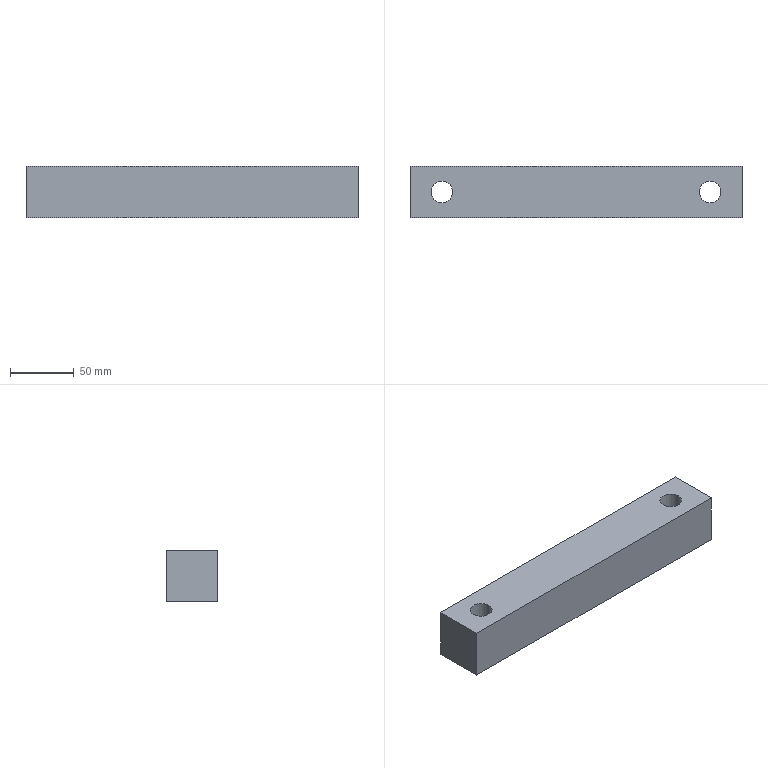Part | STEP file | 1 solid | 12 faces | box 260 x 40 x 40 mm | volume 385684 mm3 | plane 8 | cylinder 4 | commonest cylinder face diameters 17 x2 26 x2
STEP:
#1=CARTESIAN_POINT('',(3.,-262.5,-147.));
#2=VERTEX_POINT('',#1);
#3=CARTESIAN_POINT('',(-10.,-262.5,-147.));
#4=DIRECTION('',(0.,0.,-1.));
#5=DIRECTION('',(1.,0.,0.));
#6=AXIS2_PLACEMENT_3D('',#3,#4,#5);
#7=CIRCLE('',#6,13.);
#8=EDGE_CURVE('',#2,#2,#7,.T.);
#9=ORIENTED_EDGE('',*,*,#8,.F.);
#10=EDGE_LOOP('',(#9));
#11=FACE_BOUND('',#10,.T.);
#12=CARTESIAN_POINT('',(-233.,-262.5,-147.));
#13=VERTEX_POINT('',#12);
#14=CARTESIAN_POINT('',(-220.,-262.5,-147.));
#15=DIRECTION('',(0.,0.,1.));
#16=DIRECTION('',(-1.,0.,0.));
#17=AXIS2_PLACEMENT_3D('',#14,#15,#16);
#18=CIRCLE('',#17,13.);
#19=EDGE_CURVE('',#13,#13,#18,.T.);
#20=ORIENTED_EDGE('',*,*,#19,.T.);
#21=EDGE_LOOP('',(#20));
#22=FACE_BOUND('',#21,.T.);
#23=CARTESIAN_POINT('',(-245.,-282.5,-147.));
#24=VERTEX_POINT('',#23);
#25=CARTESIAN_POINT('',(15.,-282.5,-147.));
#26=VERTEX_POINT('',#25);
#27=CARTESIAN_POINT('',(25.,-282.5,-147.));
#28=DIRECTION('',(1.,0.,0.));
#29=VECTOR('',#28,1.);
#30=LINE('',#27,#29);
#31=EDGE_CURVE('',#24,#26,#30,.T.);
#32=ORIENTED_EDGE('',*,*,#31,.F.);
#33=CARTESIAN_POINT('',(-245.,-242.5,-147.));
#34=VERTEX_POINT('',#33);
#35=CARTESIAN_POINT('',(-245.,-262.5,-147.));
#36=DIRECTION('',(0.,-1.,0.));
#37=VECTOR('',#36,1.);
#38=LINE('',#35,#37);
#39=EDGE_CURVE('',#34,#24,#38,.T.);
#40=ORIENTED_EDGE('',*,*,#39,.F.);
#41=CARTESIAN_POINT('',(15.,-242.5,-147.));
#42=VERTEX_POINT('',#41);
#43=CARTESIAN_POINT('',(-22.5,-242.5,-147.));
#44=DIRECTION('',(1.,0.,0.));
#45=VECTOR('',#44,1.);
#46=LINE('',#43,#45);
#47=EDGE_CURVE('',#34,#42,#46,.T.);
#48=ORIENTED_EDGE('',*,*,#47,.T.);
#49=CARTESIAN_POINT('',(15.,-262.5,-147.));
#50=DIRECTION('',(0.,-1.,0.));
#51=VECTOR('',#50,1.);
#52=LINE('',#49,#51);
#53=EDGE_CURVE('',#42,#26,#52,.T.);
#54=ORIENTED_EDGE('',*,*,#53,.T.);
#55=EDGE_LOOP('',(#32,#40,#48,#54));
#56=FACE_BOUND('',#55,.T.);
#57=CARTESIAN_POINT('',(-115.,-262.5,-147.));
#58=DIRECTION('',(0.,0.,-1.));
#59=DIRECTION('',(-1.,0.,0.));
#60=AXIS2_PLACEMENT_3D('',#57,#58,#59);
#61=PLANE('',#60);
#62=ADVANCED_FACE('',(#11,#22,#56),#61,.T.);
#63=CARTESIAN_POINT('',(-1.5,-262.5,-107.));
#64=VERTEX_POINT('',#63);
#65=CARTESIAN_POINT('',(-10.,-262.5,-107.));
#66=DIRECTION('',(0.,0.,1.));
#67=DIRECTION('',(1.,0.,0.));
#68=AXIS2_PLACEMENT_3D('',#65,#66,#67);
#69=CIRCLE('',#68,8.5);
#70=EDGE_CURVE('',#64,#64,#69,.T.);
#71=ORIENTED_EDGE('',*,*,#70,.F.);
#72=EDGE_LOOP('',(#71));
#73=FACE_BOUND('',#72,.T.);
#74=CARTESIAN_POINT('',(-228.5,-262.5,-107.));
#75=VERTEX_POINT('',#74);
#76=CARTESIAN_POINT('',(-220.,-262.5,-107.));
#77=DIRECTION('',(0.,0.,-1.));
#78=DIRECTION('',(-1.,0.,0.));
#79=AXIS2_PLACEMENT_3D('',#76,#77,#78);
#80=CIRCLE('',#79,8.5);
#81=EDGE_CURVE('',#75,#75,#80,.T.);
#82=ORIENTED_EDGE('',*,*,#81,.T.);
#83=EDGE_LOOP('',(#82));
#84=FACE_BOUND('',#83,.T.);
#85=CARTESIAN_POINT('',(15.,-242.5,-107.));
#86=VERTEX_POINT('',#85);
#87=CARTESIAN_POINT('',(15.,-282.5,-107.));
#88=VERTEX_POINT('',#87);
#89=CARTESIAN_POINT('',(15.,9.,-107.));
#90=DIRECTION('',(0.,-1.,0.));
#91=VECTOR('',#90,1.);
#92=LINE('',#89,#91);
#93=EDGE_CURVE('',#86,#88,#92,.T.);
#94=ORIENTED_EDGE('',*,*,#93,.F.);
#95=CARTESIAN_POINT('',(-245.,-242.5,-107.));
#96=VERTEX_POINT('',#95);
#97=CARTESIAN_POINT('',(25.,-242.5,-107.));
#98=DIRECTION('',(1.,0.,0.));
#99=VECTOR('',#98,1.);
#100=LINE('',#97,#99);
#101=EDGE_CURVE('',#96,#86,#100,.T.);
#102=ORIENTED_EDGE('',*,*,#101,.F.);
#103=CARTESIAN_POINT('',(-245.,-282.5,-107.));
#104=VERTEX_POINT('',#103);
#105=CARTESIAN_POINT('',(-245.,-243.548,-107.));
#106=DIRECTION('',(0.,-1.,0.));
#107=VECTOR('',#106,1.);
#108=LINE('',#105,#107);
#109=EDGE_CURVE('',#96,#104,#108,.T.);
#110=ORIENTED_EDGE('',*,*,#109,.T.);
#111=CARTESIAN_POINT('',(25.,-282.5,-107.));
#112=DIRECTION('',(-1.,0.,0.));
#113=VECTOR('',#112,1.);
#114=LINE('',#111,#113);
#115=EDGE_CURVE('',#88,#104,#114,.T.);
#116=ORIENTED_EDGE('',*,*,#115,.F.);
#117=EDGE_LOOP('',(#94,#102,#110,#116));
#118=FACE_BOUND('',#117,.T.);
#119=CARTESIAN_POINT('',(25.,9.,-107.));
#120=DIRECTION('',(0.,0.,-1.));
#121=DIRECTION('',(0.,-1.,0.));
#122=AXIS2_PLACEMENT_3D('',#119,#120,#121);
#123=PLANE('',#122);
#124=ADVANCED_FACE('',(#73,#84,#118),#123,.F.);
#125=CARTESIAN_POINT('',(15.,-282.5,-107.));
#126=DIRECTION('',(0.,0.,1.));
#127=VECTOR('',#126,1.);
#128=LINE('',#125,#127);
#129=EDGE_CURVE('',#26,#88,#128,.T.);
#130=ORIENTED_EDGE('',*,*,#129,.F.);
#131=ORIENTED_EDGE('',*,*,#53,.F.);
#132=CARTESIAN_POINT('',(15.,-242.5,-199.5));
#133=DIRECTION('',(0.,0.,-1.));
#134=VECTOR('',#133,1.);
#135=LINE('',#132,#134);
#136=EDGE_CURVE('',#86,#42,#135,.T.);
#137=ORIENTED_EDGE('',*,*,#136,.F.);
#138=ORIENTED_EDGE('',*,*,#93,.T.);
#139=EDGE_LOOP('',(#130,#131,#137,#138));
#140=FACE_OUTER_BOUND('',#139,.T.);
#141=CARTESIAN_POINT('',(15.,9.,-107.));
#142=DIRECTION('',(-1.,0.,0.));
#143=DIRECTION('',(0.,-1.,0.));
#144=AXIS2_PLACEMENT_3D('',#141,#142,#143);
#145=PLANE('',#144);
#146=ADVANCED_FACE('',(#140),#145,.F.);
#147=ORIENTED_EDGE('',*,*,#39,.T.);
#148=CARTESIAN_POINT('',(-245.,-282.5,-107.));
#149=DIRECTION('',(0.,0.,1.));
#150=VECTOR('',#149,1.);
#151=LINE('',#148,#150);
#152=EDGE_CURVE('',#24,#104,#151,.T.);
#153=ORIENTED_EDGE('',*,*,#152,.T.);
#154=ORIENTED_EDGE('',*,*,#109,.F.);
#155=CARTESIAN_POINT('',(-245.,-242.5,-107.));
#156=DIRECTION('',(0.,0.,1.));
#157=VECTOR('',#156,1.);
#158=LINE('',#155,#157);
#159=EDGE_CURVE('',#34,#96,#158,.T.);
#160=ORIENTED_EDGE('',*,*,#159,.F.);
#161=EDGE_LOOP('',(#147,#153,#154,#160));
#162=FACE_OUTER_BOUND('',#161,.T.);
#163=CARTESIAN_POINT('',(-245.,-243.548,-107.));
#164=DIRECTION('',(1.,0.,0.));
#165=DIRECTION('',(0.,0.,1.));
#166=AXIS2_PLACEMENT_3D('',#163,#164,#165);
#167=PLANE('',#166);
#168=ADVANCED_FACE('',(#162),#167,.F.);
#169=ORIENTED_EDGE('',*,*,#152,.F.);
#170=ORIENTED_EDGE('',*,*,#31,.T.);
#171=ORIENTED_EDGE('',*,*,#129,.T.);
#172=ORIENTED_EDGE('',*,*,#115,.T.);
#173=EDGE_LOOP('',(#169,#170,#171,#172));
#174=FACE_OUTER_BOUND('',#173,.T.);
#175=CARTESIAN_POINT('',(25.,-282.5,-107.));
#176=DIRECTION('',(0.,1.,0.));
#177=DIRECTION('',(0.,0.,-1.));
#178=AXIS2_PLACEMENT_3D('',#175,#176,#177);
#179=PLANE('',#178);
#180=ADVANCED_FACE('',(#174),#179,.F.);
#181=ORIENTED_EDGE('',*,*,#136,.T.);
#182=ORIENTED_EDGE('',*,*,#47,.F.);
#183=ORIENTED_EDGE('',*,*,#159,.T.);
#184=ORIENTED_EDGE('',*,*,#101,.T.);
#185=EDGE_LOOP('',(#181,#182,#183,#184));
#186=FACE_OUTER_BOUND('',#185,.T.);
#187=CARTESIAN_POINT('',(-22.5,-242.5,-199.5));
#188=DIRECTION('',(0.,1.,0.));
#189=DIRECTION('',(0.,0.,1.));
#190=AXIS2_PLACEMENT_3D('',#187,#188,#189);
#191=PLANE('',#190);
#192=ADVANCED_FACE('',(#186),#191,.T.);
#193=CARTESIAN_POINT('',(-211.5,-262.5,-127.));
#194=VERTEX_POINT('',#193);
#195=CARTESIAN_POINT('',(-220.,-262.5,-127.));
#196=DIRECTION('',(0.,0.,1.));
#197=DIRECTION('',(1.,0.,0.));
#198=AXIS2_PLACEMENT_3D('',#195,#196,#197);
#199=CIRCLE('',#198,8.5);
#200=EDGE_CURVE('',#194,#194,#199,.T.);
#201=ORIENTED_EDGE('',*,*,#200,.F.);
#202=EDGE_LOOP('',(#201));
#203=FACE_BOUND('',#202,.T.);
#204=ORIENTED_EDGE('',*,*,#81,.F.);
#205=EDGE_LOOP('',(#204));
#206=FACE_BOUND('',#205,.T.);
#207=CARTESIAN_POINT('',(-220.,-262.5,-107.));
#208=DIRECTION('',(0.,0.,-1.));
#209=DIRECTION('',(-1.,0.,0.));
#210=AXIS2_PLACEMENT_3D('',#207,#208,#209);
#211=CYLINDRICAL_SURFACE('',#210,8.5);
#212=ADVANCED_FACE('',(#203,#206),#211,.F.);
#213=ORIENTED_EDGE('',*,*,#200,.T.);
#214=EDGE_LOOP('',(#213));
#215=FACE_BOUND('',#214,.T.);
#216=CARTESIAN_POINT('',(-233.,-262.5,-127.));
#217=VERTEX_POINT('',#216);
#218=CARTESIAN_POINT('',(-220.,-262.5,-127.));
#219=DIRECTION('',(0.,0.,1.));
#220=DIRECTION('',(-1.,0.,0.));
#221=AXIS2_PLACEMENT_3D('',#218,#219,#220);
#222=CIRCLE('',#221,13.);
#223=EDGE_CURVE('',#217,#217,#222,.T.);
#224=ORIENTED_EDGE('',*,*,#223,.F.);
#225=EDGE_LOOP('',(#224));
#226=FACE_BOUND('',#225,.T.);
#227=CARTESIAN_POINT('',(-220.,-262.5,-127.));
#228=DIRECTION('',(0.,0.,1.));
#229=DIRECTION('',(1.,0.,0.));
#230=AXIS2_PLACEMENT_3D('',#227,#228,#229);
#231=PLANE('',#230);
#232=ADVANCED_FACE('',(#215,#226),#231,.F.);
#233=ORIENTED_EDGE('',*,*,#19,.F.);
#234=EDGE_LOOP('',(#233));
#235=FACE_BOUND('',#234,.T.);
#236=ORIENTED_EDGE('',*,*,#223,.T.);
#237=EDGE_LOOP('',(#236));
#238=FACE_BOUND('',#237,.T.);
#239=CARTESIAN_POINT('',(-220.,-262.5,-127.));
#240=DIRECTION('',(0.,0.,-1.));
#241=DIRECTION('',(-1.,0.,0.));
#242=AXIS2_PLACEMENT_3D('',#239,#240,#241);
#243=CYLINDRICAL_SURFACE('',#242,13.);
#244=ADVANCED_FACE('',(#235,#238),#243,.F.);
#245=CARTESIAN_POINT('',(-18.5,-262.5,-127.));
#246=VERTEX_POINT('',#245);
#247=CARTESIAN_POINT('',(-10.,-262.5,-127.));
#248=DIRECTION('',(0.,0.,-1.));
#249=DIRECTION('',(-1.,0.,0.));
#250=AXIS2_PLACEMENT_3D('',#247,#248,#249);
#251=CIRCLE('',#250,8.5);
#252=EDGE_CURVE('',#246,#246,#251,.T.);
#253=ORIENTED_EDGE('',*,*,#252,.T.);
#254=EDGE_LOOP('',(#253));
#255=FACE_BOUND('',#254,.T.);
#256=ORIENTED_EDGE('',*,*,#70,.T.);
#257=EDGE_LOOP('',(#256));
#258=FACE_BOUND('',#257,.T.);
#259=CARTESIAN_POINT('',(-10.,-262.5,-107.));
#260=DIRECTION('',(0.,0.,-1.));
#261=DIRECTION('',(1.,0.,0.));
#262=AXIS2_PLACEMENT_3D('',#259,#260,#261);
#263=CYLINDRICAL_SURFACE('',#262,8.5);
#264=ADVANCED_FACE('',(#255,#258),#263,.F.);
#265=ORIENTED_EDGE('',*,*,#252,.F.);
#266=EDGE_LOOP('',(#265));
#267=FACE_BOUND('',#266,.T.);
#268=CARTESIAN_POINT('',(3.,-262.5,-127.));
#269=VERTEX_POINT('',#268);
#270=CARTESIAN_POINT('',(-10.,-262.5,-127.));
#271=DIRECTION('',(0.,0.,-1.));
#272=DIRECTION('',(1.,0.,0.));
#273=AXIS2_PLACEMENT_3D('',#270,#271,#272);
#274=CIRCLE('',#273,13.);
#275=EDGE_CURVE('',#269,#269,#274,.T.);
#276=ORIENTED_EDGE('',*,*,#275,.T.);
#277=EDGE_LOOP('',(#276));
#278=FACE_BOUND('',#277,.T.);
#279=CARTESIAN_POINT('',(-10.,-262.5,-127.));
#280=DIRECTION('',(0.,0.,1.));
#281=DIRECTION('',(-1.,0.,0.));
#282=AXIS2_PLACEMENT_3D('',#279,#280,#281);
#283=PLANE('',#282);
#284=ADVANCED_FACE('',(#267,#278),#283,.F.);
#285=ORIENTED_EDGE('',*,*,#8,.T.);
#286=EDGE_LOOP('',(#285));
#287=FACE_BOUND('',#286,.T.);
#288=ORIENTED_EDGE('',*,*,#275,.F.);
#289=EDGE_LOOP('',(#288));
#290=FACE_BOUND('',#289,.T.);
#291=CARTESIAN_POINT('',(-10.,-262.5,-127.));
#292=DIRECTION('',(0.,0.,-1.));
#293=DIRECTION('',(1.,0.,0.));
#294=AXIS2_PLACEMENT_3D('',#291,#292,#293);
#295=CYLINDRICAL_SURFACE('',#294,13.);
#296=ADVANCED_FACE('',(#287,#290),#295,.F.);
#297=CLOSED_SHELL('',(#62,#124,#146,#168,#180,#192,#212,#232,#244,#264,#284,#296));
#298=MANIFOLD_SOLID_BREP('',#297);
#299=(LENGTH_UNIT()NAMED_UNIT(*)SI_UNIT(.MILLI.,.METRE.));
#300=UNCERTAINTY_MEASURE_WITH_UNIT(LENGTH_MEASURE(0.00002),#299,'','');
#301=(NAMED_UNIT(*)PLANE_ANGLE_UNIT()SI_UNIT($,.RADIAN.));
#302=PLANE_ANGLE_MEASURE_WITH_UNIT(PLANE_ANGLE_MEASURE(0.01745),#301);
#303=DIMENSIONAL_EXPONENTS(0.,0.,0.,0.,0.,0.,0.);
#304=(CONVERSION_BASED_UNIT('DEGREE',#302)NAMED_UNIT(#303)PLANE_ANGLE_UNIT());
#305=(NAMED_UNIT(*)SI_UNIT($,.STERADIAN.)SOLID_ANGLE_UNIT());
#306=(GEOMETRIC_REPRESENTATION_CONTEXT(3)GLOBAL_UNCERTAINTY_ASSIGNED_CONTEXT((#300))GLOBAL_UNIT_ASSIGNED_CONTEXT((#299,#304,#305))REPRESENTATION_CONTEXT('',''));
#307=ADVANCED_BREP_SHAPE_REPRESENTATION('',(#298),#306);